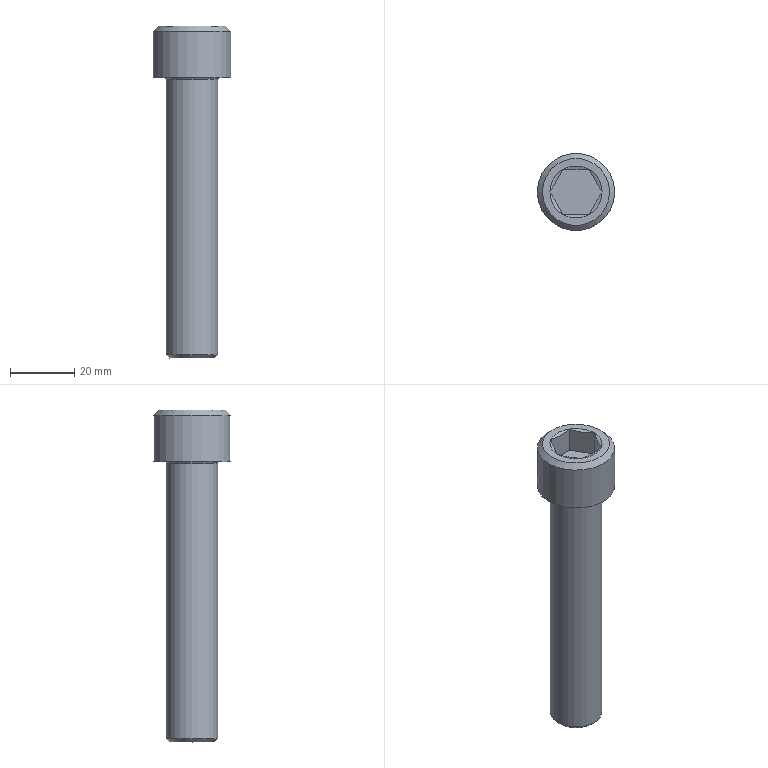Part | STEP file | solid 131 | 1 solid | 21 faces | box 24 x 24 x 103 mm | volume 23254 mm3 | plane 10 | sphere 6 | cylinder 2 | cone 2 | torus 1 | commonest cylinder face diameters 16 x1 24 x1